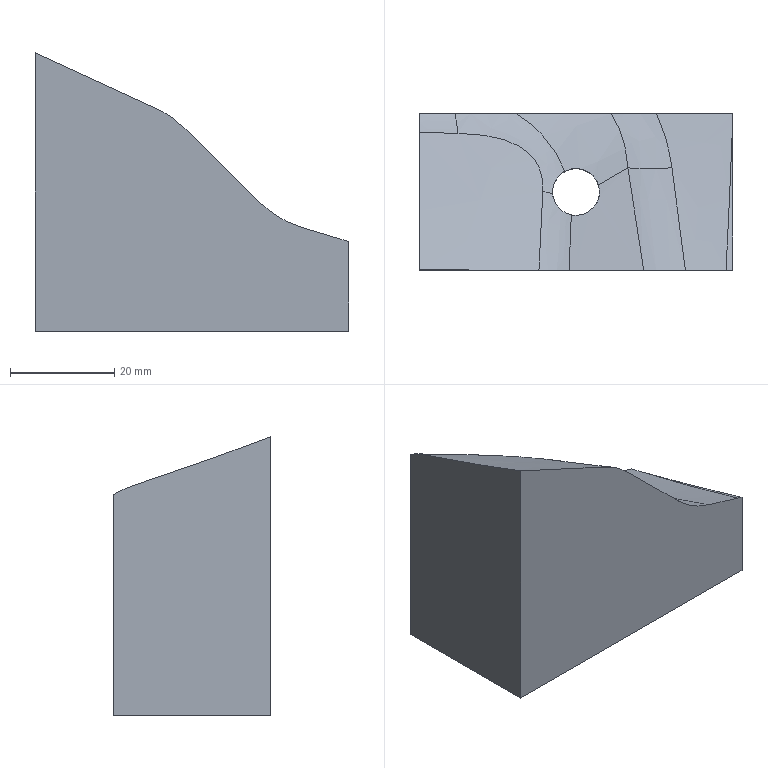Part | NX | features solid 2 | 1 solid | 16 faces | volume 51995 mm3 | spline 10 | plane 5 | cylinder 1 | commonest cylinder face diameters 9 x1